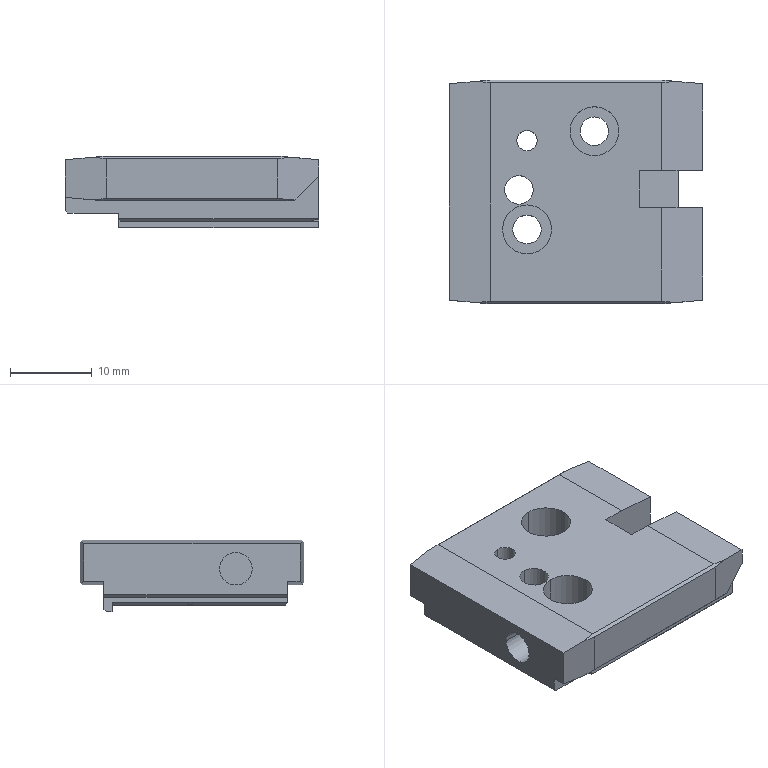Part | NX | 1 solid | 66 faces | box 31 x 27.4 x 8.8 mm | volume 5505 mm3 | plane 50 | cylinder 16 | commonest cylinder face diameters 3.5 x6 6 x4 1 x2 2.5 x2 4 x2